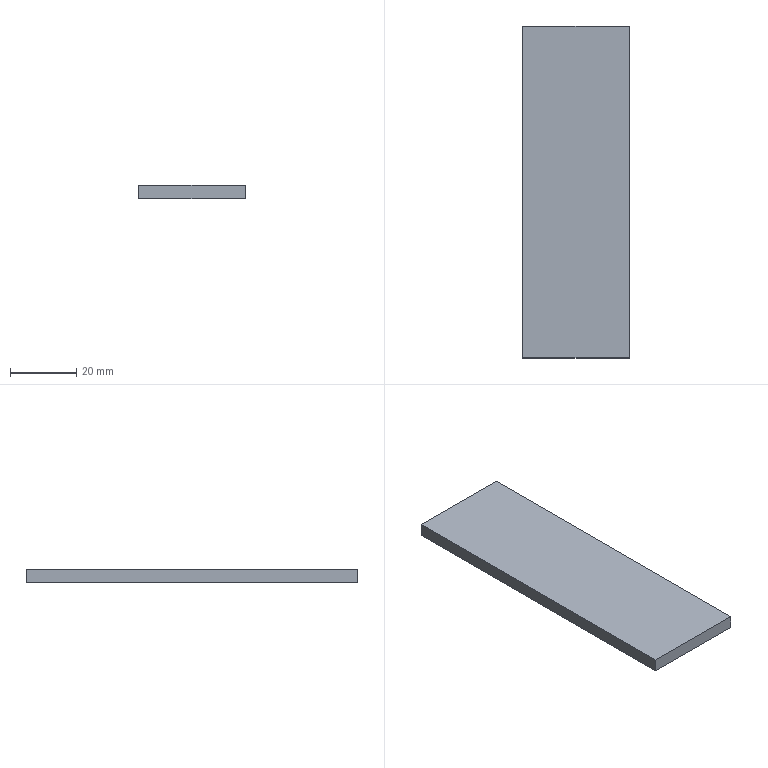Part | STEP file | X77b-01011 | 1 solid | 6 faces | box 32 x 100 x 4 mm | volume 12800 mm3 | plane 6
STEP:
#1=CARTESIAN_POINT('',(-16.,50.153,0.));
#2=VERTEX_POINT('',#1);
#3=CARTESIAN_POINT('',(-16.,-49.847,0.));
#4=VERTEX_POINT('',#3);
#5=CARTESIAN_POINT('',(-16.,50.153,0.));
#6=DIRECTION('',(0.,-1.,0.));
#7=VECTOR('',#6,1000.);
#8=LINE('',#5,#7);
#9=EDGE_CURVE('',#2,#4,#8,.T.);
#10=ORIENTED_EDGE('',*,*,#9,.T.);
#11=CARTESIAN_POINT('',(-16.,-49.847,4.));
#12=VERTEX_POINT('',#11);
#13=CARTESIAN_POINT('',(-16.,-49.847,4.));
#14=DIRECTION('',(0.,0.,-1.));
#15=VECTOR('',#14,1000.);
#16=LINE('',#13,#15);
#17=EDGE_CURVE('',#12,#4,#16,.T.);
#18=ORIENTED_EDGE('',*,*,#17,.F.);
#19=CARTESIAN_POINT('',(-16.,50.153,4.));
#20=VERTEX_POINT('',#19);
#21=CARTESIAN_POINT('',(-16.,50.153,4.));
#22=DIRECTION('',(0.,-1.,0.));
#23=VECTOR('',#22,1000.);
#24=LINE('',#21,#23);
#25=EDGE_CURVE('',#20,#12,#24,.T.);
#26=ORIENTED_EDGE('',*,*,#25,.F.);
#27=CARTESIAN_POINT('',(-16.,50.153,4.));
#28=DIRECTION('',(0.,0.,-1.));
#29=VECTOR('',#28,1000.);
#30=LINE('',#27,#29);
#31=EDGE_CURVE('',#20,#2,#30,.T.);
#32=ORIENTED_EDGE('',*,*,#31,.T.);
#33=EDGE_LOOP('',(#10,#18,#26,#32));
#34=FACE_OUTER_BOUND('',#33,.T.);
#35=CARTESIAN_POINT('',(-16.,50.153,4.));
#36=DIRECTION('',(1.,0.,0.));
#37=DIRECTION('',(0.,0.,-1.));
#38=AXIS2_PLACEMENT_3D('',#35,#36,#37);
#39=PLANE('',#38);
#40=ADVANCED_FACE('',(#34),#39,.F.);
#41=CARTESIAN_POINT('',(16.,-49.847,0.));
#42=VERTEX_POINT('',#41);
#43=CARTESIAN_POINT('',(-16.,-49.847,0.));
#44=DIRECTION('',(1.,0.,0.));
#45=VECTOR('',#44,1000.);
#46=LINE('',#43,#45);
#47=EDGE_CURVE('',#4,#42,#46,.T.);
#48=ORIENTED_EDGE('',*,*,#47,.T.);
#49=CARTESIAN_POINT('',(16.,-49.847,4.));
#50=VERTEX_POINT('',#49);
#51=CARTESIAN_POINT('',(16.,-49.847,4.));
#52=DIRECTION('',(0.,0.,-1.));
#53=VECTOR('',#52,1000.);
#54=LINE('',#51,#53);
#55=EDGE_CURVE('',#50,#42,#54,.T.);
#56=ORIENTED_EDGE('',*,*,#55,.F.);
#57=CARTESIAN_POINT('',(-16.,-49.847,4.));
#58=DIRECTION('',(1.,0.,0.));
#59=VECTOR('',#58,1000.);
#60=LINE('',#57,#59);
#61=EDGE_CURVE('',#12,#50,#60,.T.);
#62=ORIENTED_EDGE('',*,*,#61,.F.);
#63=ORIENTED_EDGE('',*,*,#17,.T.);
#64=EDGE_LOOP('',(#48,#56,#62,#63));
#65=FACE_OUTER_BOUND('',#64,.T.);
#66=CARTESIAN_POINT('',(-16.,-49.847,4.));
#67=DIRECTION('',(0.,1.,0.));
#68=DIRECTION('',(0.,0.,1.));
#69=AXIS2_PLACEMENT_3D('',#66,#67,#68);
#70=PLANE('',#69);
#71=ADVANCED_FACE('',(#65),#70,.F.);
#72=CARTESIAN_POINT('',(16.,50.153,0.));
#73=VERTEX_POINT('',#72);
#74=CARTESIAN_POINT('',(16.,50.153,0.));
#75=DIRECTION('',(0.,1.,0.));
#76=VECTOR('',#75,1000.);
#77=LINE('',#74,#76);
#78=EDGE_CURVE('',#42,#73,#77,.T.);
#79=ORIENTED_EDGE('',*,*,#78,.T.);
#80=CARTESIAN_POINT('',(16.,50.153,4.));
#81=VERTEX_POINT('',#80);
#82=CARTESIAN_POINT('',(16.,50.153,4.));
#83=DIRECTION('',(0.,0.,-1.));
#84=VECTOR('',#83,1000.);
#85=LINE('',#82,#84);
#86=EDGE_CURVE('',#81,#73,#85,.T.);
#87=ORIENTED_EDGE('',*,*,#86,.F.);
#88=CARTESIAN_POINT('',(16.,50.153,4.));
#89=DIRECTION('',(0.,1.,0.));
#90=VECTOR('',#89,1000.);
#91=LINE('',#88,#90);
#92=EDGE_CURVE('',#50,#81,#91,.T.);
#93=ORIENTED_EDGE('',*,*,#92,.F.);
#94=ORIENTED_EDGE('',*,*,#55,.T.);
#95=EDGE_LOOP('',(#79,#87,#93,#94));
#96=FACE_OUTER_BOUND('',#95,.T.);
#97=CARTESIAN_POINT('',(16.,50.153,4.));
#98=DIRECTION('',(-1.,0.,0.));
#99=DIRECTION('',(0.,0.,1.));
#100=AXIS2_PLACEMENT_3D('',#97,#98,#99);
#101=PLANE('',#100);
#102=ADVANCED_FACE('',(#96),#101,.F.);
#103=CARTESIAN_POINT('',(-16.,50.153,0.));
#104=DIRECTION('',(-1.,0.,0.));
#105=VECTOR('',#104,1000.);
#106=LINE('',#103,#105);
#107=EDGE_CURVE('',#73,#2,#106,.T.);
#108=ORIENTED_EDGE('',*,*,#107,.T.);
#109=ORIENTED_EDGE('',*,*,#31,.F.);
#110=CARTESIAN_POINT('',(-16.,50.153,4.));
#111=DIRECTION('',(-1.,0.,0.));
#112=VECTOR('',#111,1000.);
#113=LINE('',#110,#112);
#114=EDGE_CURVE('',#81,#20,#113,.T.);
#115=ORIENTED_EDGE('',*,*,#114,.F.);
#116=ORIENTED_EDGE('',*,*,#86,.T.);
#117=EDGE_LOOP('',(#108,#109,#115,#116));
#118=FACE_OUTER_BOUND('',#117,.T.);
#119=CARTESIAN_POINT('',(-16.,50.153,4.));
#120=DIRECTION('',(0.,-1.,0.));
#121=DIRECTION('',(0.,0.,-1.));
#122=AXIS2_PLACEMENT_3D('',#119,#120,#121);
#123=PLANE('',#122);
#124=ADVANCED_FACE('',(#118),#123,.F.);
#125=ORIENTED_EDGE('',*,*,#25,.T.);
#126=ORIENTED_EDGE('',*,*,#61,.T.);
#127=ORIENTED_EDGE('',*,*,#92,.T.);
#128=ORIENTED_EDGE('',*,*,#114,.T.);
#129=EDGE_LOOP('',(#125,#126,#127,#128));
#130=FACE_OUTER_BOUND('',#129,.T.);
#131=CARTESIAN_POINT('',(-16.,-49.847,4.));
#132=DIRECTION('',(0.,0.,1.));
#133=DIRECTION('',(1.,0.,0.));
#134=AXIS2_PLACEMENT_3D('',#131,#132,#133);
#135=PLANE('',#134);
#136=ADVANCED_FACE('',(#130),#135,.T.);
#137=ORIENTED_EDGE('',*,*,#9,.F.);
#138=ORIENTED_EDGE('',*,*,#107,.F.);
#139=ORIENTED_EDGE('',*,*,#78,.F.);
#140=ORIENTED_EDGE('',*,*,#47,.F.);
#141=EDGE_LOOP('',(#137,#138,#139,#140));
#142=FACE_OUTER_BOUND('',#141,.T.);
#143=CARTESIAN_POINT('',(-16.,-49.847,0.));
#144=DIRECTION('',(0.,0.,1.));
#145=DIRECTION('',(1.,0.,0.));
#146=AXIS2_PLACEMENT_3D('',#143,#144,#145);
#147=PLANE('',#146);
#148=ADVANCED_FACE('',(#142),#147,.F.);
#149=CLOSED_SHELL('',(#40,#71,#102,#124,#136,#148));
#150=MANIFOLD_SOLID_BREP('',#149);
#151=CARTESIAN_POINT('',(0.,0.,0.));
#152=DIRECTION('',(0.,0.,1.));
#153=DIRECTION('',(1.,0.,0.));
#154=AXIS2_PLACEMENT_3D('',#151,#152,#153);
#155=(LENGTH_UNIT()NAMED_UNIT(*)SI_UNIT(.MILLI.,.METRE.));
#156=UNCERTAINTY_MEASURE_WITH_UNIT(LENGTH_MEASURE(0.00001),#155,'','');
#157=(NAMED_UNIT(*)PLANE_ANGLE_UNIT()SI_UNIT($,.RADIAN.));
#158=(NAMED_UNIT(*)SI_UNIT($,.STERADIAN.)SOLID_ANGLE_UNIT());
#159=(GEOMETRIC_REPRESENTATION_CONTEXT(3)GLOBAL_UNCERTAINTY_ASSIGNED_CONTEXT((#156))GLOBAL_UNIT_ASSIGNED_CONTEXT((#155,#157,#158))REPRESENTATION_CONTEXT('',''));
#160=ADVANCED_BREP_SHAPE_REPRESENTATION('',(#150,#154),#159);